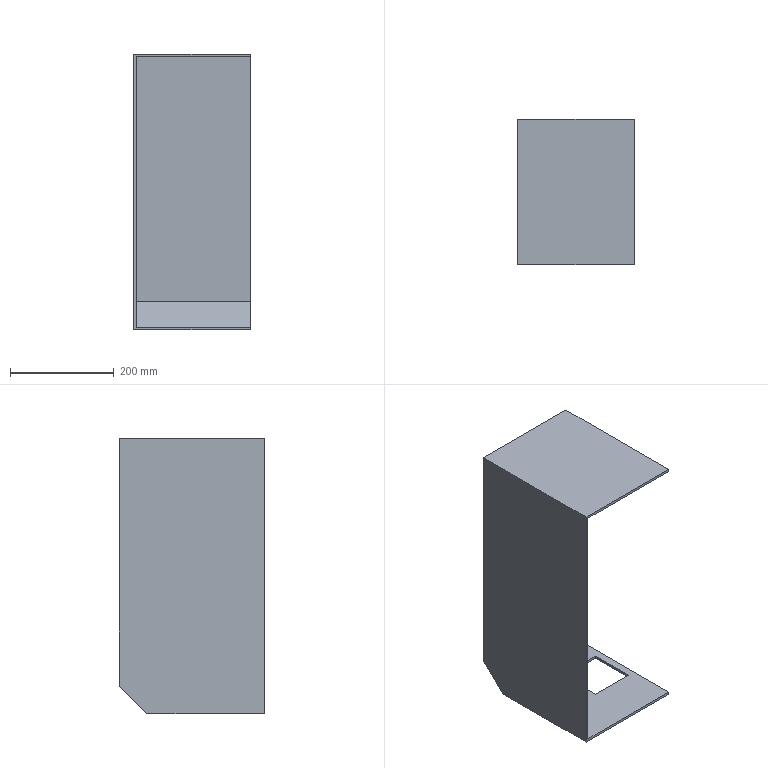Part | STEP file | Cut-Extrude 3-6 | 1 solid | 16 faces | box 225 x 280 x 530 mm | volume 1849334 mm3 | plane 16
STEP:
#1=CARTESIAN_POINT('',(-1328.738,1674.264,3043.5));
#2=VERTEX_POINT('',#1);
#3=CARTESIAN_POINT('',(-1328.738,1954.264,3043.5));
#4=VERTEX_POINT('',#3);
#5=CARTESIAN_POINT('',(-1328.738,1949.264,3043.5));
#6=DIRECTION('',(0.,1.,0.));
#7=VECTOR('',#6,1000.);
#8=LINE('',#5,#7);
#9=EDGE_CURVE('',#2,#4,#8,.T.);
#10=ORIENTED_EDGE('',*,*,#9,.T.);
#11=CARTESIAN_POINT('',(-1553.738,1954.264,3043.5));
#12=VERTEX_POINT('',#11);
#13=CARTESIAN_POINT('',(-1548.738,1954.264,3043.5));
#14=DIRECTION('',(1.,0.,0.));
#15=VECTOR('',#14,1000.);
#16=LINE('',#13,#15);
#17=EDGE_CURVE('',#12,#4,#16,.T.);
#18=ORIENTED_EDGE('',*,*,#17,.F.);
#19=CARTESIAN_POINT('',(-1553.738,1674.264,3043.5));
#20=VERTEX_POINT('',#19);
#21=CARTESIAN_POINT('',(-1553.738,1949.264,3043.5));
#22=DIRECTION('',(0.,1.,0.));
#23=VECTOR('',#22,1000.);
#24=LINE('',#21,#23);
#25=EDGE_CURVE('',#20,#12,#24,.T.);
#26=ORIENTED_EDGE('',*,*,#25,.F.);
#27=CARTESIAN_POINT('',(-1548.738,1674.264,3043.5));
#28=DIRECTION('',(1.,0.,0.));
#29=VECTOR('',#28,1000.);
#30=LINE('',#27,#29);
#31=EDGE_CURVE('',#20,#2,#30,.T.);
#32=ORIENTED_EDGE('',*,*,#31,.T.);
#33=EDGE_LOOP('',(#10,#18,#26,#32));
#34=FACE_OUTER_BOUND('',#33,.T.);
#35=CARTESIAN_POINT('',(-1548.738,1949.264,3043.5));
#36=DIRECTION('',(0.,0.,-1.));
#37=DIRECTION('',(0.,1.,0.));
#38=AXIS2_PLACEMENT_3D('',#35,#36,#37);
#39=PLANE('',#38);
#40=ADVANCED_FACE('',(#34),#39,.F.);
#41=CARTESIAN_POINT('',(-1328.738,1954.264,2566.429));
#42=VERTEX_POINT('',#41);
#43=CARTESIAN_POINT('',(-1328.738,1954.264,2518.5));
#44=DIRECTION('',(0.,0.,-1.));
#45=VECTOR('',#44,1000.);
#46=LINE('',#43,#45);
#47=EDGE_CURVE('',#4,#42,#46,.T.);
#48=ORIENTED_EDGE('',*,*,#47,.T.);
#49=CARTESIAN_POINT('',(-1553.738,1954.264,2566.429));
#50=VERTEX_POINT('',#49);
#51=CARTESIAN_POINT('',(-1548.738,1954.264,2566.429));
#52=DIRECTION('',(-1.,0.,0.));
#53=VECTOR('',#52,1000.);
#54=LINE('',#51,#53);
#55=EDGE_CURVE('',#42,#50,#54,.T.);
#56=ORIENTED_EDGE('',*,*,#55,.T.);
#57=CARTESIAN_POINT('',(-1553.738,1954.264,2518.5));
#58=DIRECTION('',(0.,0.,-1.));
#59=VECTOR('',#58,1000.);
#60=LINE('',#57,#59);
#61=EDGE_CURVE('',#12,#50,#60,.T.);
#62=ORIENTED_EDGE('',*,*,#61,.F.);
#63=ORIENTED_EDGE('',*,*,#17,.T.);
#64=EDGE_LOOP('',(#48,#56,#62,#63));
#65=FACE_OUTER_BOUND('',#64,.T.);
#66=CARTESIAN_POINT('',(-1548.738,1954.264,2518.5));
#67=DIRECTION('',(0.,-1.,0.));
#68=DIRECTION('',(0.,0.,-1.));
#69=AXIS2_PLACEMENT_3D('',#66,#67,#68);
#70=PLANE('',#69);
#71=ADVANCED_FACE('',(#65),#70,.F.);
#72=CARTESIAN_POINT('',(-1433.738,1769.264,2513.5));
#73=VERTEX_POINT('',#72);
#74=CARTESIAN_POINT('',(-1433.738,1859.264,2513.5));
#75=VERTEX_POINT('',#74);
#76=CARTESIAN_POINT('',(-1433.738,1859.264,2513.5));
#77=DIRECTION('',(0.,1.,0.));
#78=VECTOR('',#77,1000.);
#79=LINE('',#76,#78);
#80=EDGE_CURVE('',#73,#75,#79,.T.);
#81=ORIENTED_EDGE('',*,*,#80,.F.);
#82=CARTESIAN_POINT('',(-1343.738,1769.264,2513.5));
#83=VERTEX_POINT('',#82);
#84=CARTESIAN_POINT('',(-1343.738,1769.264,2513.5));
#85=DIRECTION('',(-1.,0.,0.));
#86=VECTOR('',#85,1000.);
#87=LINE('',#84,#86);
#88=EDGE_CURVE('',#83,#73,#87,.T.);
#89=ORIENTED_EDGE('',*,*,#88,.F.);
#90=CARTESIAN_POINT('',(-1343.738,1859.264,2513.5));
#91=VERTEX_POINT('',#90);
#92=CARTESIAN_POINT('',(-1343.738,1859.264,2513.5));
#93=DIRECTION('',(0.,-1.,0.));
#94=VECTOR('',#93,1000.);
#95=LINE('',#92,#94);
#96=EDGE_CURVE('',#91,#83,#95,.T.);
#97=ORIENTED_EDGE('',*,*,#96,.F.);
#98=CARTESIAN_POINT('',(-1343.738,1859.264,2513.5));
#99=DIRECTION('',(1.,0.,0.));
#100=VECTOR('',#99,1000.);
#101=LINE('',#98,#100);
#102=EDGE_CURVE('',#75,#91,#101,.T.);
#103=ORIENTED_EDGE('',*,*,#102,.F.);
#104=EDGE_LOOP('',(#81,#89,#97,#103));
#105=FACE_BOUND('',#104,.T.);
#106=CARTESIAN_POINT('',(-1553.738,1901.335,2513.5));
#107=VERTEX_POINT('',#106);
#108=CARTESIAN_POINT('',(-1553.738,1674.264,2513.5));
#109=VERTEX_POINT('',#108);
#110=CARTESIAN_POINT('',(-1553.738,1949.264,2513.5));
#111=DIRECTION('',(0.,-1.,0.));
#112=VECTOR('',#111,1000.);
#113=LINE('',#110,#112);
#114=EDGE_CURVE('',#107,#109,#113,.T.);
#115=ORIENTED_EDGE('',*,*,#114,.F.);
#116=CARTESIAN_POINT('',(-1328.738,1901.335,2513.5));
#117=VERTEX_POINT('',#116);
#118=CARTESIAN_POINT('',(-1548.738,1901.335,2513.5));
#119=DIRECTION('',(1.,0.,0.));
#120=VECTOR('',#119,1000.);
#121=LINE('',#118,#120);
#122=EDGE_CURVE('',#107,#117,#121,.T.);
#123=ORIENTED_EDGE('',*,*,#122,.T.);
#124=CARTESIAN_POINT('',(-1328.738,1674.264,2513.5));
#125=VERTEX_POINT('',#124);
#126=CARTESIAN_POINT('',(-1328.738,1949.264,2513.5));
#127=DIRECTION('',(0.,-1.,0.));
#128=VECTOR('',#127,1000.);
#129=LINE('',#126,#128);
#130=EDGE_CURVE('',#117,#125,#129,.T.);
#131=ORIENTED_EDGE('',*,*,#130,.T.);
#132=CARTESIAN_POINT('',(-1548.738,1674.264,2513.5));
#133=DIRECTION('',(1.,0.,0.));
#134=VECTOR('',#133,1000.);
#135=LINE('',#132,#134);
#136=EDGE_CURVE('',#109,#125,#135,.T.);
#137=ORIENTED_EDGE('',*,*,#136,.F.);
#138=EDGE_LOOP('',(#115,#123,#131,#137));
#139=FACE_OUTER_BOUND('',#138,.T.);
#140=CARTESIAN_POINT('',(-1548.738,1949.264,2513.5));
#141=DIRECTION('',(0.,0.,1.));
#142=DIRECTION('',(0.,-1.,0.));
#143=AXIS2_PLACEMENT_3D('',#140,#141,#142);
#144=PLANE('',#143);
#145=ADVANCED_FACE('',(#105,#139),#144,.F.);
#146=CARTESIAN_POINT('',(-1328.738,1674.264,2518.5));
#147=VERTEX_POINT('',#146);
#148=CARTESIAN_POINT('',(-1328.738,1674.264,2518.5));
#149=DIRECTION('',(0.,0.,1.));
#150=VECTOR('',#149,1000.);
#151=LINE('',#148,#150);
#152=EDGE_CURVE('',#125,#147,#151,.T.);
#153=ORIENTED_EDGE('',*,*,#152,.T.);
#154=CARTESIAN_POINT('',(-1548.738,1674.264,2518.5));
#155=VERTEX_POINT('',#154);
#156=CARTESIAN_POINT('',(-1548.738,1674.264,2518.5));
#157=DIRECTION('',(1.,0.,0.));
#158=VECTOR('',#157,1000.);
#159=LINE('',#156,#158);
#160=EDGE_CURVE('',#155,#147,#159,.T.);
#161=ORIENTED_EDGE('',*,*,#160,.F.);
#162=CARTESIAN_POINT('',(-1548.738,1674.264,3038.5));
#163=VERTEX_POINT('',#162);
#164=CARTESIAN_POINT('',(-1548.738,1674.264,2518.5));
#165=DIRECTION('',(0.,0.,-1.));
#166=VECTOR('',#165,1000.);
#167=LINE('',#164,#166);
#168=EDGE_CURVE('',#163,#155,#167,.T.);
#169=ORIENTED_EDGE('',*,*,#168,.F.);
#170=CARTESIAN_POINT('',(-1328.738,1674.264,3038.5));
#171=VERTEX_POINT('',#170);
#172=CARTESIAN_POINT('',(-1548.738,1674.264,3038.5));
#173=DIRECTION('',(-1.,0.,0.));
#174=VECTOR('',#173,1000.);
#175=LINE('',#172,#174);
#176=EDGE_CURVE('',#171,#163,#175,.T.);
#177=ORIENTED_EDGE('',*,*,#176,.F.);
#178=CARTESIAN_POINT('',(-1328.738,1674.264,2518.5));
#179=DIRECTION('',(0.,0.,1.));
#180=VECTOR('',#179,1000.);
#181=LINE('',#178,#180);
#182=EDGE_CURVE('',#171,#2,#181,.T.);
#183=ORIENTED_EDGE('',*,*,#182,.T.);
#184=ORIENTED_EDGE('',*,*,#31,.F.);
#185=CARTESIAN_POINT('',(-1553.738,1674.264,2518.5));
#186=DIRECTION('',(0.,0.,1.));
#187=VECTOR('',#186,1000.);
#188=LINE('',#185,#187);
#189=EDGE_CURVE('',#109,#20,#188,.T.);
#190=ORIENTED_EDGE('',*,*,#189,.F.);
#191=ORIENTED_EDGE('',*,*,#136,.T.);
#192=EDGE_LOOP('',(#153,#161,#169,#177,#183,#184,#190,#191));
#193=FACE_OUTER_BOUND('',#192,.T.);
#194=CARTESIAN_POINT('',(-1548.738,1674.264,2518.5));
#195=DIRECTION('',(0.,1.,0.));
#196=DIRECTION('',(0.,0.,1.));
#197=AXIS2_PLACEMENT_3D('',#194,#195,#196);
#198=PLANE('',#197);
#199=ADVANCED_FACE('',(#193),#198,.F.);
#200=ORIENTED_EDGE('',*,*,#61,.T.);
#201=CARTESIAN_POINT('',(-1553.738,1990.3,2602.464));
#202=DIRECTION('',(0.,-0.7071,-0.7071));
#203=VECTOR('',#202,1000.);
#204=LINE('',#201,#203);
#205=EDGE_CURVE('',#50,#107,#204,.T.);
#206=ORIENTED_EDGE('',*,*,#205,.T.);
#207=ORIENTED_EDGE('',*,*,#114,.T.);
#208=ORIENTED_EDGE('',*,*,#189,.T.);
#209=ORIENTED_EDGE('',*,*,#25,.T.);
#210=EDGE_LOOP('',(#200,#206,#207,#208,#209));
#211=FACE_OUTER_BOUND('',#210,.T.);
#212=CARTESIAN_POINT('',(-1553.738,1814.264,2778.5));
#213=DIRECTION('',(-1.,0.,0.));
#214=DIRECTION('',(0.,1.,0.));
#215=AXIS2_PLACEMENT_3D('',#212,#213,#214);
#216=PLANE('',#215);
#217=ADVANCED_FACE('',(#211),#216,.T.);
#218=CARTESIAN_POINT('',(-1328.738,1899.264,2518.5));
#219=VERTEX_POINT('',#218);
#220=CARTESIAN_POINT('',(-1328.738,1949.264,2518.5));
#221=DIRECTION('',(0.,-1.,0.));
#222=VECTOR('',#221,1000.);
#223=LINE('',#220,#222);
#224=EDGE_CURVE('',#219,#147,#223,.T.);
#225=ORIENTED_EDGE('',*,*,#224,.T.);
#226=ORIENTED_EDGE('',*,*,#152,.F.);
#227=ORIENTED_EDGE('',*,*,#130,.F.);
#228=CARTESIAN_POINT('',(-1328.738,1902.8,2514.964));
#229=DIRECTION('',(0.,0.7071,0.7071));
#230=VECTOR('',#229,1000.);
#231=LINE('',#228,#230);
#232=EDGE_CURVE('',#117,#42,#231,.T.);
#233=ORIENTED_EDGE('',*,*,#232,.T.);
#234=ORIENTED_EDGE('',*,*,#47,.F.);
#235=ORIENTED_EDGE('',*,*,#9,.F.);
#236=ORIENTED_EDGE('',*,*,#182,.F.);
#237=CARTESIAN_POINT('',(-1328.738,1949.264,3038.5));
#238=VERTEX_POINT('',#237);
#239=CARTESIAN_POINT('',(-1328.738,1949.264,3038.5));
#240=DIRECTION('',(0.,1.,0.));
#241=VECTOR('',#240,1000.);
#242=LINE('',#239,#241);
#243=EDGE_CURVE('',#171,#238,#242,.T.);
#244=ORIENTED_EDGE('',*,*,#243,.T.);
#245=CARTESIAN_POINT('',(-1328.738,1949.264,2568.5));
#246=VERTEX_POINT('',#245);
#247=CARTESIAN_POINT('',(-1328.738,1949.264,2518.5));
#248=DIRECTION('',(0.,0.,-1.));
#249=VECTOR('',#248,1000.);
#250=LINE('',#247,#249);
#251=EDGE_CURVE('',#238,#246,#250,.T.);
#252=ORIENTED_EDGE('',*,*,#251,.T.);
#253=CARTESIAN_POINT('',(-1328.738,1899.264,2518.5));
#254=DIRECTION('',(0.,0.7071,0.7071));
#255=VECTOR('',#254,1000.);
#256=LINE('',#253,#255);
#257=EDGE_CURVE('',#219,#246,#256,.T.);
#258=ORIENTED_EDGE('',*,*,#257,.F.);
#259=EDGE_LOOP('',(#225,#226,#227,#233,#234,#235,#236,#244,#252,#258));
#260=FACE_OUTER_BOUND('',#259,.T.);
#261=CARTESIAN_POINT('',(-1328.738,1814.264,2778.5));
#262=DIRECTION('',(-1.,0.,0.));
#263=DIRECTION('',(0.,1.,0.));
#264=AXIS2_PLACEMENT_3D('',#261,#262,#263);
#265=PLANE('',#264);
#266=ADVANCED_FACE('',(#260),#265,.F.);
#267=ORIENTED_EDGE('',*,*,#205,.F.);
#268=ORIENTED_EDGE('',*,*,#55,.F.);
#269=ORIENTED_EDGE('',*,*,#232,.F.);
#270=ORIENTED_EDGE('',*,*,#122,.F.);
#271=EDGE_LOOP('',(#267,#268,#269,#270));
#272=FACE_OUTER_BOUND('',#271,.T.);
#273=CARTESIAN_POINT('',(-1548.738,1902.8,2514.964));
#274=DIRECTION('',(0.,-0.7071,0.7071));
#275=DIRECTION('',(-1.,0.,0.));
#276=AXIS2_PLACEMENT_3D('',#273,#274,#275);
#277=PLANE('',#276);
#278=ADVANCED_FACE('',(#272),#277,.F.);
#279=CARTESIAN_POINT('',(-1548.738,1949.264,3038.5));
#280=VERTEX_POINT('',#279);
#281=CARTESIAN_POINT('',(-1548.738,1949.264,3038.5));
#282=DIRECTION('',(0.,1.,0.));
#283=VECTOR('',#282,1000.);
#284=LINE('',#281,#283);
#285=EDGE_CURVE('',#163,#280,#284,.T.);
#286=ORIENTED_EDGE('',*,*,#285,.T.);
#287=CARTESIAN_POINT('',(-1548.738,1949.264,3038.5));
#288=DIRECTION('',(1.,0.,0.));
#289=VECTOR('',#288,1000.);
#290=LINE('',#287,#289);
#291=EDGE_CURVE('',#280,#238,#290,.T.);
#292=ORIENTED_EDGE('',*,*,#291,.T.);
#293=ORIENTED_EDGE('',*,*,#243,.F.);
#294=ORIENTED_EDGE('',*,*,#176,.T.);
#295=EDGE_LOOP('',(#286,#292,#293,#294));
#296=FACE_OUTER_BOUND('',#295,.T.);
#297=CARTESIAN_POINT('',(-1548.738,1949.264,3038.5));
#298=DIRECTION('',(0.,0.,-1.));
#299=DIRECTION('',(0.,1.,0.));
#300=AXIS2_PLACEMENT_3D('',#297,#298,#299);
#301=PLANE('',#300);
#302=ADVANCED_FACE('',(#296),#301,.T.);
#303=ORIENTED_EDGE('',*,*,#251,.F.);
#304=ORIENTED_EDGE('',*,*,#291,.F.);
#305=CARTESIAN_POINT('',(-1548.738,1949.264,2568.5));
#306=VERTEX_POINT('',#305);
#307=CARTESIAN_POINT('',(-1548.738,1949.264,2518.5));
#308=DIRECTION('',(0.,0.,-1.));
#309=VECTOR('',#308,1000.);
#310=LINE('',#307,#309);
#311=EDGE_CURVE('',#280,#306,#310,.T.);
#312=ORIENTED_EDGE('',*,*,#311,.T.);
#313=CARTESIAN_POINT('',(-1548.738,1949.264,2568.5));
#314=DIRECTION('',(-1.,0.,0.));
#315=VECTOR('',#314,1000.);
#316=LINE('',#313,#315);
#317=EDGE_CURVE('',#246,#306,#316,.T.);
#318=ORIENTED_EDGE('',*,*,#317,.F.);
#319=EDGE_LOOP('',(#303,#304,#312,#318));
#320=FACE_OUTER_BOUND('',#319,.T.);
#321=CARTESIAN_POINT('',(-1548.738,1949.264,2518.5));
#322=DIRECTION('',(0.,-1.,0.));
#323=DIRECTION('',(0.,0.,-1.));
#324=AXIS2_PLACEMENT_3D('',#321,#322,#323);
#325=PLANE('',#324);
#326=ADVANCED_FACE('',(#320),#325,.T.);
#327=ORIENTED_EDGE('',*,*,#160,.T.);
#328=ORIENTED_EDGE('',*,*,#224,.F.);
#329=CARTESIAN_POINT('',(-1548.738,1899.264,2518.5));
#330=VERTEX_POINT('',#329);
#331=CARTESIAN_POINT('',(-1548.738,1899.264,2518.5));
#332=DIRECTION('',(1.,0.,0.));
#333=VECTOR('',#332,1000.);
#334=LINE('',#331,#333);
#335=EDGE_CURVE('',#330,#219,#334,.T.);
#336=ORIENTED_EDGE('',*,*,#335,.F.);
#337=CARTESIAN_POINT('',(-1548.738,1949.264,2518.5));
#338=DIRECTION('',(0.,-1.,0.));
#339=VECTOR('',#338,1000.);
#340=LINE('',#337,#339);
#341=EDGE_CURVE('',#330,#155,#340,.T.);
#342=ORIENTED_EDGE('',*,*,#341,.T.);
#343=EDGE_LOOP('',(#327,#328,#336,#342));
#344=FACE_OUTER_BOUND('',#343,.T.);
#345=CARTESIAN_POINT('',(-1433.738,1769.264,2518.5));
#346=VERTEX_POINT('',#345);
#347=CARTESIAN_POINT('',(-1343.738,1769.264,2518.5));
#348=VERTEX_POINT('',#347);
#349=CARTESIAN_POINT('',(-1548.738,1769.264,2518.5));
#350=DIRECTION('',(1.,0.,0.));
#351=VECTOR('',#350,1000.);
#352=LINE('',#349,#351);
#353=EDGE_CURVE('',#346,#348,#352,.T.);
#354=ORIENTED_EDGE('',*,*,#353,.F.);
#355=CARTESIAN_POINT('',(-1433.738,1859.264,2518.5));
#356=VERTEX_POINT('',#355);
#357=CARTESIAN_POINT('',(-1433.738,1949.264,2518.5));
#358=DIRECTION('',(0.,-1.,0.));
#359=VECTOR('',#358,1000.);
#360=LINE('',#357,#359);
#361=EDGE_CURVE('',#356,#346,#360,.T.);
#362=ORIENTED_EDGE('',*,*,#361,.F.);
#363=CARTESIAN_POINT('',(-1343.738,1859.264,2518.5));
#364=VERTEX_POINT('',#363);
#365=CARTESIAN_POINT('',(-1548.738,1859.264,2518.5));
#366=DIRECTION('',(-1.,0.,0.));
#367=VECTOR('',#366,1000.);
#368=LINE('',#365,#367);
#369=EDGE_CURVE('',#364,#356,#368,.T.);
#370=ORIENTED_EDGE('',*,*,#369,.F.);
#371=CARTESIAN_POINT('',(-1343.738,1949.264,2518.5));
#372=DIRECTION('',(0.,1.,0.));
#373=VECTOR('',#372,1000.);
#374=LINE('',#371,#373);
#375=EDGE_CURVE('',#348,#364,#374,.T.);
#376=ORIENTED_EDGE('',*,*,#375,.F.);
#377=EDGE_LOOP('',(#354,#362,#370,#376));
#378=FACE_BOUND('',#377,.T.);
#379=CARTESIAN_POINT('',(-1548.738,1949.264,2518.5));
#380=DIRECTION('',(0.,0.,1.));
#381=DIRECTION('',(0.,-1.,0.));
#382=AXIS2_PLACEMENT_3D('',#379,#380,#381);
#383=PLANE('',#382);
#384=ADVANCED_FACE('',(#344,#378),#383,.T.);
#385=ORIENTED_EDGE('',*,*,#168,.T.);
#386=ORIENTED_EDGE('',*,*,#341,.F.);
#387=CARTESIAN_POINT('',(-1548.738,1986.764,2606.));
#388=DIRECTION('',(0.,-0.7071,-0.7071));
#389=VECTOR('',#388,1000.);
#390=LINE('',#387,#389);
#391=EDGE_CURVE('',#306,#330,#390,.T.);
#392=ORIENTED_EDGE('',*,*,#391,.F.);
#393=ORIENTED_EDGE('',*,*,#311,.F.);
#394=ORIENTED_EDGE('',*,*,#285,.F.);
#395=EDGE_LOOP('',(#385,#386,#392,#393,#394));
#396=FACE_OUTER_BOUND('',#395,.T.);
#397=CARTESIAN_POINT('',(-1548.738,1814.264,2778.5));
#398=DIRECTION('',(-1.,0.,0.));
#399=DIRECTION('',(0.,1.,0.));
#400=AXIS2_PLACEMENT_3D('',#397,#398,#399);
#401=PLANE('',#400);
#402=ADVANCED_FACE('',(#396),#401,.F.);
#403=ORIENTED_EDGE('',*,*,#391,.T.);
#404=ORIENTED_EDGE('',*,*,#335,.T.);
#405=ORIENTED_EDGE('',*,*,#257,.T.);
#406=ORIENTED_EDGE('',*,*,#317,.T.);
#407=EDGE_LOOP('',(#403,#404,#405,#406));
#408=FACE_OUTER_BOUND('',#407,.T.);
#409=CARTESIAN_POINT('',(-1548.738,1899.264,2518.5));
#410=DIRECTION('',(0.,-0.7071,0.7071));
#411=DIRECTION('',(-1.,0.,0.));
#412=AXIS2_PLACEMENT_3D('',#409,#410,#411);
#413=PLANE('',#412);
#414=ADVANCED_FACE('',(#408),#413,.T.);
#415=ORIENTED_EDGE('',*,*,#353,.T.);
#416=CARTESIAN_POINT('',(-1343.738,1769.264,2525.5));
#417=DIRECTION('',(0.,0.,-1.));
#418=VECTOR('',#417,1000.);
#419=LINE('',#416,#418);
#420=EDGE_CURVE('',#348,#83,#419,.T.);
#421=ORIENTED_EDGE('',*,*,#420,.T.);
#422=ORIENTED_EDGE('',*,*,#88,.T.);
#423=CARTESIAN_POINT('',(-1433.738,1769.264,2525.5));
#424=DIRECTION('',(0.,0.,-1.));
#425=VECTOR('',#424,1000.);
#426=LINE('',#423,#425);
#427=EDGE_CURVE('',#346,#73,#426,.T.);
#428=ORIENTED_EDGE('',*,*,#427,.F.);
#429=EDGE_LOOP('',(#415,#421,#422,#428));
#430=FACE_OUTER_BOUND('',#429,.T.);
#431=CARTESIAN_POINT('',(-1343.738,1769.264,2525.5));
#432=DIRECTION('',(0.,-1.,0.));
#433=DIRECTION('',(0.,0.,-1.));
#434=AXIS2_PLACEMENT_3D('',#431,#432,#433);
#435=PLANE('',#434);
#436=ADVANCED_FACE('',(#430),#435,.F.);
#437=ORIENTED_EDGE('',*,*,#375,.T.);
#438=CARTESIAN_POINT('',(-1343.738,1859.264,2525.5));
#439=DIRECTION('',(0.,0.,-1.));
#440=VECTOR('',#439,1000.);
#441=LINE('',#438,#440);
#442=EDGE_CURVE('',#364,#91,#441,.T.);
#443=ORIENTED_EDGE('',*,*,#442,.T.);
#444=ORIENTED_EDGE('',*,*,#96,.T.);
#445=ORIENTED_EDGE('',*,*,#420,.F.);
#446=EDGE_LOOP('',(#437,#443,#444,#445));
#447=FACE_OUTER_BOUND('',#446,.T.);
#448=CARTESIAN_POINT('',(-1343.738,1859.264,2525.5));
#449=DIRECTION('',(1.,0.,0.));
#450=DIRECTION('',(0.,-1.,0.));
#451=AXIS2_PLACEMENT_3D('',#448,#449,#450);
#452=PLANE('',#451);
#453=ADVANCED_FACE('',(#447),#452,.F.);
#454=ORIENTED_EDGE('',*,*,#369,.T.);
#455=CARTESIAN_POINT('',(-1433.738,1859.264,2525.5));
#456=DIRECTION('',(0.,0.,-1.));
#457=VECTOR('',#456,1000.);
#458=LINE('',#455,#457);
#459=EDGE_CURVE('',#356,#75,#458,.T.);
#460=ORIENTED_EDGE('',*,*,#459,.T.);
#461=ORIENTED_EDGE('',*,*,#102,.T.);
#462=ORIENTED_EDGE('',*,*,#442,.F.);
#463=EDGE_LOOP('',(#454,#460,#461,#462));
#464=FACE_OUTER_BOUND('',#463,.T.);
#465=CARTESIAN_POINT('',(-1343.738,1859.264,2525.5));
#466=DIRECTION('',(0.,1.,0.));
#467=DIRECTION('',(0.,0.,1.));
#468=AXIS2_PLACEMENT_3D('',#465,#466,#467);
#469=PLANE('',#468);
#470=ADVANCED_FACE('',(#464),#469,.F.);
#471=ORIENTED_EDGE('',*,*,#361,.T.);
#472=ORIENTED_EDGE('',*,*,#427,.T.);
#473=ORIENTED_EDGE('',*,*,#80,.T.);
#474=ORIENTED_EDGE('',*,*,#459,.F.);
#475=EDGE_LOOP('',(#471,#472,#473,#474));
#476=FACE_OUTER_BOUND('',#475,.T.);
#477=CARTESIAN_POINT('',(-1433.738,1859.264,2525.5));
#478=DIRECTION('',(-1.,0.,0.));
#479=DIRECTION('',(0.,1.,0.));
#480=AXIS2_PLACEMENT_3D('',#477,#478,#479);
#481=PLANE('',#480);
#482=ADVANCED_FACE('',(#476),#481,.F.);
#483=CLOSED_SHELL('',(#40,#71,#145,#199,#217,#266,#278,#302,#326,#384,#402,#414,#436,#453,#470,#482));
#484=MANIFOLD_SOLID_BREP('',#483);
#485=CARTESIAN_POINT('',(0.,0.,0.));
#486=DIRECTION('',(0.,0.,1.));
#487=DIRECTION('',(1.,0.,0.));
#488=AXIS2_PLACEMENT_3D('',#485,#486,#487);
#489=(LENGTH_UNIT()NAMED_UNIT(*)SI_UNIT(.MILLI.,.METRE.));
#490=UNCERTAINTY_MEASURE_WITH_UNIT(LENGTH_MEASURE(0.00001),#489,'','');
#491=(NAMED_UNIT(*)PLANE_ANGLE_UNIT()SI_UNIT($,.RADIAN.));
#492=(NAMED_UNIT(*)SI_UNIT($,.STERADIAN.)SOLID_ANGLE_UNIT());
#493=(GEOMETRIC_REPRESENTATION_CONTEXT(3)GLOBAL_UNCERTAINTY_ASSIGNED_CONTEXT((#490))GLOBAL_UNIT_ASSIGNED_CONTEXT((#489,#491,#492))REPRESENTATION_CONTEXT('',''));
#494=ADVANCED_BREP_SHAPE_REPRESENTATION('',(#484,#488),#493);